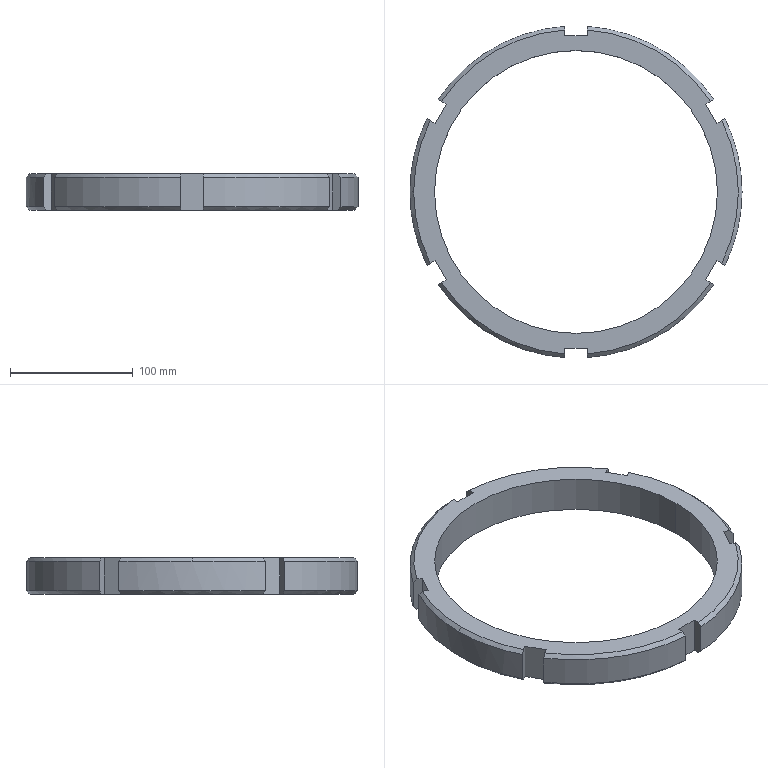Part | SolidWorks | features Chamfer 1, CirPattern 1, ICE 1, Revolution 1 | 1 solid | 43 faces | box 270 x 269.399 x 30 mm | volume 439038 mm3 | plane 20 | cone 14 | cylinder 9 | commonest cylinder face diameters 270 x7 230 x2
STEP:
#1=CARTESIAN_POINT('',(-115.,0.,-30.));
#2=VERTEX_POINT('',#1);
#3=CARTESIAN_POINT('',(115.,0.,-30.));
#4=VERTEX_POINT('',#3);
#5=CARTESIAN_POINT('',(0.,0.,-30.));
#6=DIRECTION('',(0.,0.,1.));
#7=DIRECTION('',(1.,0.,0.));
#8=AXIS2_PLACEMENT_3D('',#5,#6,#7);
#9=CIRCLE('',#8,115.);
#10=EDGE_CURVE('',#2,#4,#9,.T.);
#11=ORIENTED_EDGE('',*,*,#10,.F.);
#12=CARTESIAN_POINT('',(-115.,0.,0.));
#13=VERTEX_POINT('',#12);
#14=CARTESIAN_POINT('',(-115.,0.,0.));
#15=DIRECTION('',(0.,0.,1.));
#16=VECTOR('',#15,1000.);
#17=LINE('',#14,#16);
#18=EDGE_CURVE('',#2,#13,#17,.T.);
#19=ORIENTED_EDGE('',*,*,#18,.T.);
#20=CARTESIAN_POINT('',(115.,0.,0.));
#21=VERTEX_POINT('',#20);
#22=CARTESIAN_POINT('',(0.,0.,0.));
#23=DIRECTION('',(0.,0.,1.));
#24=DIRECTION('',(1.,0.,0.));
#25=AXIS2_PLACEMENT_3D('',#22,#23,#24);
#26=CIRCLE('',#25,115.);
#27=EDGE_CURVE('',#13,#21,#26,.T.);
#28=ORIENTED_EDGE('',*,*,#27,.T.);
#29=CARTESIAN_POINT('',(115.,0.,0.));
#30=DIRECTION('',(0.,0.,1.));
#31=VECTOR('',#30,1000.);
#32=LINE('',#29,#31);
#33=EDGE_CURVE('',#4,#21,#32,.T.);
#34=ORIENTED_EDGE('',*,*,#33,.F.);
#35=EDGE_LOOP('',(#11,#19,#28,#34));
#36=FACE_OUTER_BOUND('',#35,.T.);
#37=CARTESIAN_POINT('',(0.,0.,0.));
#38=DIRECTION('',(0.,0.,1.));
#39=DIRECTION('',(1.,0.,0.));
#40=AXIS2_PLACEMENT_3D('',#37,#38,#39);
#41=CYLINDRICAL_SURFACE('',#40,115.);
#42=ADVANCED_FACE('',(#36),#41,.F.);
#43=CARTESIAN_POINT('',(-132.,0.,0.));
#44=VERTEX_POINT('',#43);
#45=CARTESIAN_POINT('',(-118.549,-58.052,0.));
#46=VERTEX_POINT('',#45);
#47=CARTESIAN_POINT('',(0.,0.,0.));
#48=DIRECTION('',(0.,0.,1.));
#49=DIRECTION('',(-1.,0.,0.));
#50=AXIS2_PLACEMENT_3D('',#47,#48,#49);
#51=CIRCLE('',#50,132.);
#52=EDGE_CURVE('',#44,#46,#51,.T.);
#53=ORIENTED_EDGE('',*,*,#52,.F.);
#54=CARTESIAN_POINT('',(-135.,0.,-3.));
#55=VERTEX_POINT('',#54);
#56=CARTESIAN_POINT('',(-132.,0.,0.));
#57=DIRECTION('',(-0.7071,0.,-0.7071));
#58=VECTOR('',#57,1000.);
#59=LINE('',#56,#58);
#60=EDGE_CURVE('',#44,#55,#59,.T.);
#61=ORIENTED_EDGE('',*,*,#60,.T.);
#62=CARTESIAN_POINT('',(-121.153,-59.556,-3.));
#63=VERTEX_POINT('',#62);
#64=CARTESIAN_POINT('',(0.,0.,-3.));
#65=DIRECTION('',(0.,0.,-1.));
#66=DIRECTION('',(-1.,0.,0.));
#67=AXIS2_PLACEMENT_3D('',#64,#65,#66);
#68=CIRCLE('',#67,135.);
#69=EDGE_CURVE('',#63,#55,#68,.T.);
#70=ORIENTED_EDGE('',*,*,#69,.F.);
#71=CARTESIAN_POINT('',(-118.549,-58.052,0.));
#72=CARTESIAN_POINT('',(-119.417,-58.553,-1.));
#73=CARTESIAN_POINT('',(-120.285,-59.054,-2.));
#74=CARTESIAN_POINT('',(-121.153,-59.556,-3.));
#75=B_SPLINE_CURVE_WITH_KNOTS('',3,(#71,#72,#73,#74),.UNSPECIFIED.,.F.,.F.,(4,4),(0.000000283,0.004248),.UNSPECIFIED.);
#76=EDGE_CURVE('',#46,#63,#75,.T.);
#77=ORIENTED_EDGE('',*,*,#76,.F.);
#78=EDGE_LOOP('',(#53,#61,#70,#77));
#79=FACE_OUTER_BOUND('',#78,.T.);
#80=CARTESIAN_POINT('',(0.,0.,0.));
#81=DIRECTION('',(0.,0.,-1.));
#82=DIRECTION('',(-1.,0.,0.));
#83=AXIS2_PLACEMENT_3D('',#80,#81,#82);
#84=CONICAL_SURFACE('',#83,132.,0.7854);
#85=ADVANCED_FACE('',(#79),#84,.T.);
#86=CARTESIAN_POINT('',(132.,0.,-30.));
#87=VERTEX_POINT('',#86);
#88=CARTESIAN_POINT('',(118.549,-58.052,-30.));
#89=VERTEX_POINT('',#88);
#90=CARTESIAN_POINT('',(0.,0.,-30.));
#91=DIRECTION('',(0.,0.,-1.));
#92=DIRECTION('',(1.,0.,0.));
#93=AXIS2_PLACEMENT_3D('',#90,#91,#92);
#94=CIRCLE('',#93,132.);
#95=EDGE_CURVE('',#87,#89,#94,.T.);
#96=ORIENTED_EDGE('',*,*,#95,.F.);
#97=CARTESIAN_POINT('',(135.,0.,-27.));
#98=VERTEX_POINT('',#97);
#99=CARTESIAN_POINT('',(135.,0.,-27.));
#100=DIRECTION('',(0.7071,0.,0.7071));
#101=VECTOR('',#100,1000.);
#102=LINE('',#99,#101);
#103=EDGE_CURVE('',#87,#98,#102,.T.);
#104=ORIENTED_EDGE('',*,*,#103,.T.);
#105=CARTESIAN_POINT('',(121.153,-59.556,-27.));
#106=VERTEX_POINT('',#105);
#107=CARTESIAN_POINT('',(0.,0.,-27.));
#108=DIRECTION('',(0.,0.,1.));
#109=DIRECTION('',(1.,0.,0.));
#110=AXIS2_PLACEMENT_3D('',#107,#108,#109);
#111=CIRCLE('',#110,135.);
#112=EDGE_CURVE('',#106,#98,#111,.T.);
#113=ORIENTED_EDGE('',*,*,#112,.F.);
#114=CARTESIAN_POINT('',(118.549,-58.052,-30.));
#115=CARTESIAN_POINT('',(119.417,-58.553,-29.));
#116=CARTESIAN_POINT('',(120.285,-59.054,-28.));
#117=CARTESIAN_POINT('',(121.153,-59.556,-27.));
#118=B_SPLINE_CURVE_WITH_KNOTS('',3,(#114,#115,#116,#117),.UNSPECIFIED.,.F.,.F.,(4,4),(0.000000283,0.004248),.UNSPECIFIED.);
#119=EDGE_CURVE('',#89,#106,#118,.T.);
#120=ORIENTED_EDGE('',*,*,#119,.F.);
#121=EDGE_LOOP('',(#96,#104,#113,#120));
#122=FACE_OUTER_BOUND('',#121,.T.);
#123=CARTESIAN_POINT('',(0.,0.,-27.));
#124=DIRECTION('',(0.,0.,1.));
#125=DIRECTION('',(1.,0.,0.));
#126=AXIS2_PLACEMENT_3D('',#123,#124,#125);
#127=CONICAL_SURFACE('',#126,135.,0.7854);
#128=ADVANCED_FACE('',(#122),#127,.T.);
#129=ORIENTED_EDGE('',*,*,#112,.T.);
#130=CARTESIAN_POINT('',(135.,0.,-3.));
#131=VERTEX_POINT('',#130);
#132=CARTESIAN_POINT('',(135.,0.,0.));
#133=DIRECTION('',(0.,0.,1.));
#134=VECTOR('',#133,1000.);
#135=LINE('',#132,#134);
#136=EDGE_CURVE('',#98,#131,#135,.T.);
#137=ORIENTED_EDGE('',*,*,#136,.T.);
#138=CARTESIAN_POINT('',(121.153,-59.556,-3.));
#139=VERTEX_POINT('',#138);
#140=CARTESIAN_POINT('',(0.,0.,-3.));
#141=DIRECTION('',(0.,0.,-1.));
#142=DIRECTION('',(-1.,0.,0.));
#143=AXIS2_PLACEMENT_3D('',#140,#141,#142);
#144=CIRCLE('',#143,135.);
#145=EDGE_CURVE('',#131,#139,#144,.T.);
#146=ORIENTED_EDGE('',*,*,#145,.T.);
#147=CARTESIAN_POINT('',(121.153,-59.556,0.));
#148=DIRECTION('',(0.,0.,-1.));
#149=VECTOR('',#148,1000.);
#150=LINE('',#147,#149);
#151=EDGE_CURVE('',#139,#106,#150,.T.);
#152=ORIENTED_EDGE('',*,*,#151,.T.);
#153=EDGE_LOOP('',(#129,#137,#146,#152));
#154=FACE_OUTER_BOUND('',#153,.T.);
#155=CARTESIAN_POINT('',(0.,0.,0.));
#156=DIRECTION('',(0.,0.,1.));
#157=DIRECTION('',(1.,0.,0.));
#158=AXIS2_PLACEMENT_3D('',#155,#156,#157);
#159=CYLINDRICAL_SURFACE('',#158,135.);
#160=ADVANCED_FACE('',(#154),#159,.T.);
#161=CARTESIAN_POINT('',(-9.,-134.7,-3.));
#162=VERTEX_POINT('',#161);
#163=CARTESIAN_POINT('',(-112.153,-75.144,-3.));
#164=VERTEX_POINT('',#163);
#165=CARTESIAN_POINT('',(0.,0.,-3.));
#166=DIRECTION('',(0.,0.,-1.));
#167=DIRECTION('',(-1.,0.,0.));
#168=AXIS2_PLACEMENT_3D('',#165,#166,#167);
#169=CIRCLE('',#168,135.);
#170=EDGE_CURVE('',#162,#164,#169,.T.);
#171=ORIENTED_EDGE('',*,*,#170,.T.);
#172=CARTESIAN_POINT('',(-112.153,-75.144,-27.));
#173=VERTEX_POINT('',#172);
#174=CARTESIAN_POINT('',(-112.153,-75.144,0.));
#175=DIRECTION('',(0.,0.,-1.));
#176=VECTOR('',#175,1000.);
#177=LINE('',#174,#176);
#178=EDGE_CURVE('',#164,#173,#177,.T.);
#179=ORIENTED_EDGE('',*,*,#178,.T.);
#180=CARTESIAN_POINT('',(-9.,-134.7,-27.));
#181=VERTEX_POINT('',#180);
#182=CARTESIAN_POINT('',(0.,0.,-27.));
#183=DIRECTION('',(0.,0.,1.));
#184=DIRECTION('',(1.,0.,0.));
#185=AXIS2_PLACEMENT_3D('',#182,#183,#184);
#186=CIRCLE('',#185,135.);
#187=EDGE_CURVE('',#173,#181,#186,.T.);
#188=ORIENTED_EDGE('',*,*,#187,.T.);
#189=CARTESIAN_POINT('',(-9.,-134.7,0.));
#190=DIRECTION('',(0.,0.,1.));
#191=VECTOR('',#190,1000.);
#192=LINE('',#189,#191);
#193=EDGE_CURVE('',#181,#162,#192,.T.);
#194=ORIENTED_EDGE('',*,*,#193,.T.);
#195=EDGE_LOOP('',(#171,#179,#188,#194));
#196=FACE_OUTER_BOUND('',#195,.T.);
#197=CARTESIAN_POINT('',(0.,0.,0.));
#198=DIRECTION('',(0.,0.,1.));
#199=DIRECTION('',(1.,0.,0.));
#200=AXIS2_PLACEMENT_3D('',#197,#198,#199);
#201=CYLINDRICAL_SURFACE('',#200,135.);
#202=ADVANCED_FACE('',(#196),#201,.T.);
#203=CARTESIAN_POINT('',(112.153,-75.144,-3.));
#204=VERTEX_POINT('',#203);
#205=CARTESIAN_POINT('',(9.,-134.7,-3.));
#206=VERTEX_POINT('',#205);
#207=CARTESIAN_POINT('',(0.,0.,-3.));
#208=DIRECTION('',(0.,0.,-1.));
#209=DIRECTION('',(-1.,0.,0.));
#210=AXIS2_PLACEMENT_3D('',#207,#208,#209);
#211=CIRCLE('',#210,135.);
#212=EDGE_CURVE('',#204,#206,#211,.T.);
#213=ORIENTED_EDGE('',*,*,#212,.T.);
#214=CARTESIAN_POINT('',(9.,-134.7,-27.));
#215=VERTEX_POINT('',#214);
#216=CARTESIAN_POINT('',(9.,-134.7,0.));
#217=DIRECTION('',(0.,0.,-1.));
#218=VECTOR('',#217,1000.);
#219=LINE('',#216,#218);
#220=EDGE_CURVE('',#206,#215,#219,.T.);
#221=ORIENTED_EDGE('',*,*,#220,.T.);
#222=CARTESIAN_POINT('',(112.153,-75.144,-27.));
#223=VERTEX_POINT('',#222);
#224=CARTESIAN_POINT('',(0.,0.,-27.));
#225=DIRECTION('',(0.,0.,1.));
#226=DIRECTION('',(1.,0.,0.));
#227=AXIS2_PLACEMENT_3D('',#224,#225,#226);
#228=CIRCLE('',#227,135.);
#229=EDGE_CURVE('',#215,#223,#228,.T.);
#230=ORIENTED_EDGE('',*,*,#229,.T.);
#231=CARTESIAN_POINT('',(112.153,-75.144,0.));
#232=DIRECTION('',(0.,0.,1.));
#233=VECTOR('',#232,1000.);
#234=LINE('',#231,#233);
#235=EDGE_CURVE('',#223,#204,#234,.T.);
#236=ORIENTED_EDGE('',*,*,#235,.T.);
#237=EDGE_LOOP('',(#213,#221,#230,#236));
#238=FACE_OUTER_BOUND('',#237,.T.);
#239=CARTESIAN_POINT('',(0.,0.,0.));
#240=DIRECTION('',(0.,0.,1.));
#241=DIRECTION('',(1.,0.,0.));
#242=AXIS2_PLACEMENT_3D('',#239,#240,#241);
#243=CYLINDRICAL_SURFACE('',#242,135.);
#244=ADVANCED_FACE('',(#238),#243,.T.);
#245=ORIENTED_EDGE('',*,*,#136,.F.);
#246=CARTESIAN_POINT('',(121.153,59.556,-27.));
#247=VERTEX_POINT('',#246);
#248=CARTESIAN_POINT('',(0.,0.,-27.));
#249=DIRECTION('',(0.,0.,1.));
#250=DIRECTION('',(1.,0.,0.));
#251=AXIS2_PLACEMENT_3D('',#248,#249,#250);
#252=CIRCLE('',#251,135.);
#253=EDGE_CURVE('',#98,#247,#252,.T.);
#254=ORIENTED_EDGE('',*,*,#253,.T.);
#255=CARTESIAN_POINT('',(121.153,59.556,-3.));
#256=VERTEX_POINT('',#255);
#257=CARTESIAN_POINT('',(121.153,59.556,0.));
#258=DIRECTION('',(0.,0.,1.));
#259=VECTOR('',#258,1000.);
#260=LINE('',#257,#259);
#261=EDGE_CURVE('',#247,#256,#260,.T.);
#262=ORIENTED_EDGE('',*,*,#261,.T.);
#263=CARTESIAN_POINT('',(0.,0.,-3.));
#264=DIRECTION('',(0.,0.,-1.));
#265=DIRECTION('',(-1.,0.,0.));
#266=AXIS2_PLACEMENT_3D('',#263,#264,#265);
#267=CIRCLE('',#266,135.);
#268=EDGE_CURVE('',#256,#131,#267,.T.);
#269=ORIENTED_EDGE('',*,*,#268,.T.);
#270=EDGE_LOOP('',(#245,#254,#262,#269));
#271=FACE_OUTER_BOUND('',#270,.T.);
#272=CARTESIAN_POINT('',(0.,0.,0.));
#273=DIRECTION('',(0.,0.,1.));
#274=DIRECTION('',(1.,0.,0.));
#275=AXIS2_PLACEMENT_3D('',#272,#273,#274);
#276=CYLINDRICAL_SURFACE('',#275,135.);
#277=ADVANCED_FACE('',(#271),#276,.T.);
#278=CARTESIAN_POINT('',(9.,134.7,-3.));
#279=VERTEX_POINT('',#278);
#280=CARTESIAN_POINT('',(112.153,75.144,-3.));
#281=VERTEX_POINT('',#280);
#282=CARTESIAN_POINT('',(0.,0.,-3.));
#283=DIRECTION('',(0.,0.,-1.));
#284=DIRECTION('',(-1.,0.,0.));
#285=AXIS2_PLACEMENT_3D('',#282,#283,#284);
#286=CIRCLE('',#285,135.);
#287=EDGE_CURVE('',#279,#281,#286,.T.);
#288=ORIENTED_EDGE('',*,*,#287,.T.);
#289=CARTESIAN_POINT('',(112.153,75.144,-27.));
#290=VERTEX_POINT('',#289);
#291=CARTESIAN_POINT('',(112.153,75.144,0.));
#292=DIRECTION('',(0.,0.,-1.));
#293=VECTOR('',#292,1000.);
#294=LINE('',#291,#293);
#295=EDGE_CURVE('',#281,#290,#294,.T.);
#296=ORIENTED_EDGE('',*,*,#295,.T.);
#297=CARTESIAN_POINT('',(9.,134.7,-27.));
#298=VERTEX_POINT('',#297);
#299=CARTESIAN_POINT('',(0.,0.,-27.));
#300=DIRECTION('',(0.,0.,1.));
#301=DIRECTION('',(1.,0.,0.));
#302=AXIS2_PLACEMENT_3D('',#299,#300,#301);
#303=CIRCLE('',#302,135.);
#304=EDGE_CURVE('',#290,#298,#303,.T.);
#305=ORIENTED_EDGE('',*,*,#304,.T.);
#306=CARTESIAN_POINT('',(9.,134.7,0.));
#307=DIRECTION('',(0.,0.,1.));
#308=VECTOR('',#307,1000.);
#309=LINE('',#306,#308);
#310=EDGE_CURVE('',#298,#279,#309,.T.);
#311=ORIENTED_EDGE('',*,*,#310,.T.);
#312=EDGE_LOOP('',(#288,#296,#305,#311));
#313=FACE_OUTER_BOUND('',#312,.T.);
#314=CARTESIAN_POINT('',(0.,0.,0.));
#315=DIRECTION('',(0.,0.,1.));
#316=DIRECTION('',(1.,0.,0.));
#317=AXIS2_PLACEMENT_3D('',#314,#315,#316);
#318=CYLINDRICAL_SURFACE('',#317,135.);
#319=ADVANCED_FACE('',(#313),#318,.T.);
#320=CARTESIAN_POINT('',(-109.549,-73.641,-30.));
#321=VERTEX_POINT('',#320);
#322=CARTESIAN_POINT('',(-109.549,-73.641,-30.));
#323=CARTESIAN_POINT('',(-110.417,-74.142,-29.));
#324=CARTESIAN_POINT('',(-111.285,-74.643,-28.));
#325=CARTESIAN_POINT('',(-112.153,-75.144,-27.));
#326=B_SPLINE_CURVE_WITH_KNOTS('',3,(#322,#323,#324,#325),.UNSPECIFIED.,.F.,.F.,(4,4),(0.000000283,0.004248),.UNSPECIFIED.);
#327=EDGE_CURVE('',#321,#173,#326,.T.);
#328=ORIENTED_EDGE('',*,*,#327,.F.);
#329=CARTESIAN_POINT('',(-9.,-131.693,-30.));
#330=VERTEX_POINT('',#329);
#331=CARTESIAN_POINT('',(0.,0.,-30.));
#332=DIRECTION('',(0.,0.,-1.));
#333=DIRECTION('',(1.,0.,0.));
#334=AXIS2_PLACEMENT_3D('',#331,#332,#333);
#335=CIRCLE('',#334,132.);
#336=EDGE_CURVE('',#330,#321,#335,.T.);
#337=ORIENTED_EDGE('',*,*,#336,.F.);
#338=CARTESIAN_POINT('',(-9.,-134.7,-27.));
#339=CARTESIAN_POINT('',(-9.,-134.333,-27.366));
#340=CARTESIAN_POINT('',(-9.,-133.966,-27.732));
#341=CARTESIAN_POINT('',(-9.,-133.599,-28.098));
#342=CARTESIAN_POINT('',(-9.,-132.964,-28.732));
#343=CARTESIAN_POINT('',(-9.,-132.328,-29.366));
#344=CARTESIAN_POINT('',(-9.,-131.693,-30.));
#345=B_SPLINE_CURVE_WITH_KNOTS('',3,(#338,#339,#340,#341,#342,#343,#344),.UNSPECIFIED.,.F.,.F.,(4,3,4),(0.01543,0.01698,0.01967),.UNSPECIFIED.);
#346=EDGE_CURVE('',#181,#330,#345,.T.);
#347=ORIENTED_EDGE('',*,*,#346,.F.);
#348=ORIENTED_EDGE('',*,*,#187,.F.);
#349=EDGE_LOOP('',(#328,#337,#347,#348));
#350=FACE_OUTER_BOUND('',#349,.T.);
#351=CARTESIAN_POINT('',(0.,0.,-27.));
#352=DIRECTION('',(0.,0.,1.));
#353=DIRECTION('',(1.,0.,0.));
#354=AXIS2_PLACEMENT_3D('',#351,#352,#353);
#355=CONICAL_SURFACE('',#354,135.,0.7854);
#356=ADVANCED_FACE('',(#350),#355,.T.);
#357=CARTESIAN_POINT('',(9.,-131.693,-30.));
#358=VERTEX_POINT('',#357);
#359=CARTESIAN_POINT('',(9.,-131.693,-30.));
#360=CARTESIAN_POINT('',(9.,-132.328,-29.366));
#361=CARTESIAN_POINT('',(9.,-132.964,-28.732));
#362=CARTESIAN_POINT('',(9.,-133.599,-28.098));
#363=CARTESIAN_POINT('',(9.,-133.966,-27.732));
#364=CARTESIAN_POINT('',(9.,-134.333,-27.366));
#365=CARTESIAN_POINT('',(9.,-134.7,-27.));
#366=B_SPLINE_CURVE_WITH_KNOTS('',3,(#359,#360,#361,#362,#363,#364,#365),.UNSPECIFIED.,.F.,.F.,(4,3,4),(0.01429,0.01698,0.01854),.UNSPECIFIED.);
#367=EDGE_CURVE('',#358,#215,#366,.T.);
#368=ORIENTED_EDGE('',*,*,#367,.F.);
#369=CARTESIAN_POINT('',(109.549,-73.641,-30.));
#370=VERTEX_POINT('',#369);
#371=CARTESIAN_POINT('',(0.,0.,-30.));
#372=DIRECTION('',(0.,0.,-1.));
#373=DIRECTION('',(1.,0.,0.));
#374=AXIS2_PLACEMENT_3D('',#371,#372,#373);
#375=CIRCLE('',#374,132.);
#376=EDGE_CURVE('',#370,#358,#375,.T.);
#377=ORIENTED_EDGE('',*,*,#376,.F.);
#378=CARTESIAN_POINT('',(112.153,-75.144,-27.));
#379=CARTESIAN_POINT('',(111.285,-74.643,-28.));
#380=CARTESIAN_POINT('',(110.417,-74.142,-29.));
#381=CARTESIAN_POINT('',(109.549,-73.641,-30.));
#382=B_SPLINE_CURVE_WITH_KNOTS('',3,(#378,#379,#380,#381),.UNSPECIFIED.,.F.,.F.,(4,4),(0.000000283,0.004248),.UNSPECIFIED.);
#383=EDGE_CURVE('',#223,#370,#382,.T.);
#384=ORIENTED_EDGE('',*,*,#383,.F.);
#385=ORIENTED_EDGE('',*,*,#229,.F.);
#386=EDGE_LOOP('',(#368,#377,#384,#385));
#387=FACE_OUTER_BOUND('',#386,.T.);
#388=CARTESIAN_POINT('',(0.,0.,-27.));
#389=DIRECTION('',(0.,0.,1.));
#390=DIRECTION('',(1.,0.,0.));
#391=AXIS2_PLACEMENT_3D('',#388,#389,#390);
#392=CONICAL_SURFACE('',#391,135.,0.7854);
#393=ADVANCED_FACE('',(#387),#392,.T.);
#394=ORIENTED_EDGE('',*,*,#103,.F.);
#395=CARTESIAN_POINT('',(118.549,58.052,-30.));
#396=VERTEX_POINT('',#395);
#397=CARTESIAN_POINT('',(0.,0.,-30.));
#398=DIRECTION('',(0.,0.,-1.));
#399=DIRECTION('',(1.,0.,0.));
#400=AXIS2_PLACEMENT_3D('',#397,#398,#399);
#401=CIRCLE('',#400,132.);
#402=EDGE_CURVE('',#396,#87,#401,.T.);
#403=ORIENTED_EDGE('',*,*,#402,.F.);
#404=CARTESIAN_POINT('',(121.153,59.556,-27.));
#405=CARTESIAN_POINT('',(120.285,59.054,-28.));
#406=CARTESIAN_POINT('',(119.417,58.553,-29.));
#407=CARTESIAN_POINT('',(118.549,58.052,-30.));
#408=B_SPLINE_CURVE_WITH_KNOTS('',3,(#404,#405,#406,#407),.UNSPECIFIED.,.F.,.F.,(4,4),(0.000000283,0.004248),.UNSPECIFIED.);
#409=EDGE_CURVE('',#247,#396,#408,.T.);
#410=ORIENTED_EDGE('',*,*,#409,.F.);
#411=ORIENTED_EDGE('',*,*,#253,.F.);
#412=EDGE_LOOP('',(#394,#403,#410,#411));
#413=FACE_OUTER_BOUND('',#412,.T.);
#414=CARTESIAN_POINT('',(0.,0.,-27.));
#415=DIRECTION('',(0.,0.,1.));
#416=DIRECTION('',(1.,0.,0.));
#417=AXIS2_PLACEMENT_3D('',#414,#415,#416);
#418=CONICAL_SURFACE('',#417,135.,0.7854);
#419=ADVANCED_FACE('',(#413),#418,.T.);
#420=CARTESIAN_POINT('',(109.549,73.641,-30.));
#421=VERTEX_POINT('',#420);
#422=CARTESIAN_POINT('',(109.549,73.641,-30.));
#423=CARTESIAN_POINT('',(110.417,74.142,-29.));
#424=CARTESIAN_POINT('',(111.285,74.643,-28.));
#425=CARTESIAN_POINT('',(112.153,75.144,-27.));
#426=B_SPLINE_CURVE_WITH_KNOTS('',3,(#422,#423,#424,#425),.UNSPECIFIED.,.F.,.F.,(4,4),(0.000000283,0.004248),.UNSPECIFIED.);
#427=EDGE_CURVE('',#421,#290,#426,.T.);
#428=ORIENTED_EDGE('',*,*,#427,.F.);
#429=CARTESIAN_POINT('',(9.,131.693,-30.));
#430=VERTEX_POINT('',#429);
#431=CARTESIAN_POINT('',(0.,0.,-30.));
#432=DIRECTION('',(0.,0.,-1.));
#433=DIRECTION('',(1.,0.,0.));
#434=AXIS2_PLACEMENT_3D('',#431,#432,#433);
#435=CIRCLE('',#434,132.);
#436=EDGE_CURVE('',#430,#421,#435,.T.);
#437=ORIENTED_EDGE('',*,*,#436,.F.);
#438=CARTESIAN_POINT('',(9.,134.7,-27.));
#439=CARTESIAN_POINT('',(9.,133.999,-27.699));
#440=CARTESIAN_POINT('',(9.,133.298,-28.399));
#441=CARTESIAN_POINT('',(9.,132.597,-29.098));
#442=CARTESIAN_POINT('',(9.,132.295,-29.399));
#443=CARTESIAN_POINT('',(9.,131.994,-29.699));
#444=CARTESIAN_POINT('',(9.,131.693,-30.));
#445=B_SPLINE_CURVE_WITH_KNOTS('',3,(#438,#439,#440,#441,#442,#443,#444),.UNSPECIFIED.,.F.,.F.,(4,3,4),(0.01401,0.01698,0.01826),.UNSPECIFIED.);
#446=EDGE_CURVE('',#298,#430,#445,.T.);
#447=ORIENTED_EDGE('',*,*,#446,.F.);
#448=ORIENTED_EDGE('',*,*,#304,.F.);
#449=EDGE_LOOP('',(#428,#437,#447,#448));
#450=FACE_OUTER_BOUND('',#449,.T.);
#451=CARTESIAN_POINT('',(0.,0.,-27.));
#452=DIRECTION('',(0.,0.,1.));
#453=DIRECTION('',(1.,0.,0.));
#454=AXIS2_PLACEMENT_3D('',#451,#452,#453);
#455=CONICAL_SURFACE('',#454,135.,0.7854);
#456=ADVANCED_FACE('',(#450),#455,.T.);
#457=CARTESIAN_POINT('',(-109.549,-73.641,0.));
#458=VERTEX_POINT('',#457);
#459=CARTESIAN_POINT('',(-112.153,-75.144,-3.));
#460=CARTESIAN_POINT('',(-111.285,-74.643,-2.));
#461=CARTESIAN_POINT('',(-110.417,-74.142,-1.));
#462=CARTESIAN_POINT('',(-109.549,-73.641,0.));
#463=B_SPLINE_CURVE_WITH_KNOTS('',3,(#459,#460,#461,#462),.UNSPECIFIED.,.F.,.F.,(4,4),(0.000000283,0.004248),.UNSPECIFIED.);
#464=EDGE_CURVE('',#164,#458,#463,.T.);
#465=ORIENTED_EDGE('',*,*,#464,.F.);
#466=ORIENTED_EDGE('',*,*,#170,.F.);
#467=CARTESIAN_POINT('',(-9.,-131.693,0.));
#468=VERTEX_POINT('',#467);
#469=CARTESIAN_POINT('',(-9.,-131.693,0.));
#470=CARTESIAN_POINT('',(-9.,-132.328,-0.6339));
#471=CARTESIAN_POINT('',(-9.,-132.964,-1.268));
#472=CARTESIAN_POINT('',(-9.,-133.599,-1.902));
#473=CARTESIAN_POINT('',(-9.,-133.966,-2.268));
#474=CARTESIAN_POINT('',(-9.,-134.333,-2.634));
#475=CARTESIAN_POINT('',(-9.,-134.7,-3.));
#476=B_SPLINE_CURVE_WITH_KNOTS('',3,(#469,#470,#471,#472,#473,#474,#475),.UNSPECIFIED.,.F.,.F.,(4,3,4),(0.01429,0.01698,0.01854),.UNSPECIFIED.);
#477=EDGE_CURVE('',#468,#162,#476,.T.);
#478=ORIENTED_EDGE('',*,*,#477,.F.);
#479=CARTESIAN_POINT('',(0.,0.,0.));
#480=DIRECTION('',(0.,0.,1.));
#481=DIRECTION('',(-1.,0.,0.));
#482=AXIS2_PLACEMENT_3D('',#479,#480,#481);
#483=CIRCLE('',#482,132.);
#484=EDGE_CURVE('',#458,#468,#483,.T.);
#485=ORIENTED_EDGE('',*,*,#484,.F.);
#486=EDGE_LOOP('',(#465,#466,#478,#485));
#487=FACE_OUTER_BOUND('',#486,.T.);
#488=CARTESIAN_POINT('',(0.,0.,0.));
#489=DIRECTION('',(0.,0.,-1.));
#490=DIRECTION('',(-1.,0.,0.));
#491=AXIS2_PLACEMENT_3D('',#488,#489,#490);
#492=CONICAL_SURFACE('',#491,132.,0.7854);
#493=ADVANCED_FACE('',(#487),#492,.T.);
#494=CARTESIAN_POINT('',(9.,-131.693,0.));
#495=VERTEX_POINT('',#494);
#496=CARTESIAN_POINT('',(9.,-134.7,-3.));
#497=CARTESIAN_POINT('',(9.,-134.333,-2.634));
#498=CARTESIAN_POINT('',(9.,-133.966,-2.268));
#499=CARTESIAN_POINT('',(9.,-133.599,-1.902));
#500=CARTESIAN_POINT('',(9.,-132.964,-1.268));
#501=CARTESIAN_POINT('',(9.,-132.328,-0.6339));
#502=CARTESIAN_POINT('',(9.,-131.693,0.));
#503=B_SPLINE_CURVE_WITH_KNOTS('',3,(#496,#497,#498,#499,#500,#501,#502),.UNSPECIFIED.,.F.,.F.,(4,3,4),(0.01543,0.01698,0.01967),.UNSPECIFIED.);
#504=EDGE_CURVE('',#206,#495,#503,.T.);
#505=ORIENTED_EDGE('',*,*,#504,.F.);
#506=ORIENTED_EDGE('',*,*,#212,.F.);
#507=CARTESIAN_POINT('',(109.549,-73.641,0.));
#508=VERTEX_POINT('',#507);
#509=CARTESIAN_POINT('',(109.549,-73.641,0.));
#510=CARTESIAN_POINT('',(110.417,-74.142,-1.));
#511=CARTESIAN_POINT('',(111.285,-74.643,-2.));
#512=CARTESIAN_POINT('',(112.153,-75.144,-3.));
#513=B_SPLINE_CURVE_WITH_KNOTS('',3,(#509,#510,#511,#512),.UNSPECIFIED.,.F.,.F.,(4,4),(0.000000283,0.004248),.UNSPECIFIED.);
#514=EDGE_CURVE('',#508,#204,#513,.T.);
#515=ORIENTED_EDGE('',*,*,#514,.F.);
#516=CARTESIAN_POINT('',(0.,0.,0.));
#517=DIRECTION('',(0.,0.,1.));
#518=DIRECTION('',(-1.,0.,0.));
#519=AXIS2_PLACEMENT_3D('',#516,#517,#518);
#520=CIRCLE('',#519,132.);
#521=EDGE_CURVE('',#495,#508,#520,.T.);
#522=ORIENTED_EDGE('',*,*,#521,.F.);
#523=EDGE_LOOP('',(#505,#506,#515,#522));
#524=FACE_OUTER_BOUND('',#523,.T.);
#525=CARTESIAN_POINT('',(0.,0.,0.));
#526=DIRECTION('',(0.,0.,-1.));
#527=DIRECTION('',(-1.,0.,0.));
#528=AXIS2_PLACEMENT_3D('',#525,#526,#527);
#529=CONICAL_SURFACE('',#528,132.,0.7854);
#530=ADVANCED_FACE('',(#524),#529,.T.);
#531=CARTESIAN_POINT('',(118.549,-58.052,0.));
#532=VERTEX_POINT('',#531);
#533=CARTESIAN_POINT('',(121.153,-59.556,-3.));
#534=CARTESIAN_POINT('',(120.285,-59.054,-2.));
#535=CARTESIAN_POINT('',(119.417,-58.553,-1.));
#536=CARTESIAN_POINT('',(118.549,-58.052,0.));
#537=B_SPLINE_CURVE_WITH_KNOTS('',3,(#533,#534,#535,#536),.UNSPECIFIED.,.F.,.F.,(4,4),(0.000000283,0.004248),.UNSPECIFIED.);
#538=EDGE_CURVE('',#139,#532,#537,.T.);
#539=ORIENTED_EDGE('',*,*,#538,.F.);
#540=ORIENTED_EDGE('',*,*,#145,.F.);
#541=ORIENTED_EDGE('',*,*,#268,.F.);
#542=CARTESIAN_POINT('',(118.549,58.052,0.));
#543=VERTEX_POINT('',#542);
#544=CARTESIAN_POINT('',(118.549,58.052,0.));
#545=CARTESIAN_POINT('',(119.417,58.553,-1.));
#546=CARTESIAN_POINT('',(120.285,59.054,-2.));
#547=CARTESIAN_POINT('',(121.153,59.556,-3.));
#548=B_SPLINE_CURVE_WITH_KNOTS('',3,(#544,#545,#546,#547),.UNSPECIFIED.,.F.,.F.,(4,4),(0.000000283,0.004248),.UNSPECIFIED.);
#549=EDGE_CURVE('',#543,#256,#548,.T.);
#550=ORIENTED_EDGE('',*,*,#549,.F.);
#551=CARTESIAN_POINT('',(0.,0.,0.));
#552=DIRECTION('',(0.,0.,1.));
#553=DIRECTION('',(-1.,0.,0.));
#554=AXIS2_PLACEMENT_3D('',#551,#552,#553);
#555=CIRCLE('',#554,132.);
#556=EDGE_CURVE('',#532,#543,#555,.T.);
#557=ORIENTED_EDGE('',*,*,#556,.F.);
#558=EDGE_LOOP('',(#539,#540,#541,#550,#557));
#559=FACE_OUTER_BOUND('',#558,.T.);
#560=CARTESIAN_POINT('',(0.,0.,0.));
#561=DIRECTION('',(0.,0.,-1.));
#562=DIRECTION('',(-1.,0.,0.));
#563=AXIS2_PLACEMENT_3D('',#560,#561,#562);
#564=CONICAL_SURFACE('',#563,132.,0.7854);
#565=ADVANCED_FACE('',(#559),#564,.T.);
#566=CARTESIAN_POINT('',(109.549,73.641,0.));
#567=VERTEX_POINT('',#566);
#568=CARTESIAN_POINT('',(112.153,75.144,-3.));
#569=CARTESIAN_POINT('',(111.285,74.643,-2.));
#570=CARTESIAN_POINT('',(110.417,74.142,-1.));
#571=CARTESIAN_POINT('',(109.549,73.641,0.));
#572=B_SPLINE_CURVE_WITH_KNOTS('',3,(#568,#569,#570,#571),.UNSPECIFIED.,.F.,.F.,(4,4),(0.000000283,0.004248),.UNSPECIFIED.);
#573=EDGE_CURVE('',#281,#567,#572,.T.);
#574=ORIENTED_EDGE('',*,*,#573,.F.);
#575=ORIENTED_EDGE('',*,*,#287,.F.);
#576=CARTESIAN_POINT('',(9.,131.693,0.));
#577=VERTEX_POINT('',#576);
#578=CARTESIAN_POINT('',(9.,131.693,0.));
#579=CARTESIAN_POINT('',(9.,131.994,-0.3006));
#580=CARTESIAN_POINT('',(9.,132.295,-0.6012));
#581=CARTESIAN_POINT('',(9.,132.597,-0.9019));
#582=CARTESIAN_POINT('',(9.,133.298,-1.601));
#583=CARTESIAN_POINT('',(9.,133.999,-2.301));
#584=CARTESIAN_POINT('',(9.,134.7,-3.));
#585=B_SPLINE_CURVE_WITH_KNOTS('',3,(#578,#579,#580,#581,#582,#583,#584),.UNSPECIFIED.,.F.,.F.,(4,3,4),(0.0157,0.01698,0.01995),.UNSPECIFIED.);
#586=EDGE_CURVE('',#577,#279,#585,.T.);
#587=ORIENTED_EDGE('',*,*,#586,.F.);
#588=CARTESIAN_POINT('',(0.,0.,0.));
#589=DIRECTION('',(0.,0.,1.));
#590=DIRECTION('',(-1.,0.,0.));
#591=AXIS2_PLACEMENT_3D('',#588,#589,#590);
#592=CIRCLE('',#591,132.);
#593=EDGE_CURVE('',#567,#577,#592,.T.);
#594=ORIENTED_EDGE('',*,*,#593,.F.);
#595=EDGE_LOOP('',(#574,#575,#587,#594));
#596=FACE_OUTER_BOUND('',#595,.T.);
#597=CARTESIAN_POINT('',(0.,0.,0.));
#598=DIRECTION('',(0.,0.,-1.));
#599=DIRECTION('',(-1.,0.,0.));
#600=AXIS2_PLACEMENT_3D('',#597,#598,#599);
#601=CONICAL_SURFACE('',#600,132.,0.7854);
#602=ADVANCED_FACE('',(#596),#601,.T.);
#603=CARTESIAN_POINT('',(-121.153,59.556,-27.));
#604=VERTEX_POINT('',#603);
#605=CARTESIAN_POINT('',(-121.153,-59.556,-27.));
#606=VERTEX_POINT('',#605);
#607=CARTESIAN_POINT('',(0.,0.,-27.));
#608=DIRECTION('',(0.,0.,1.));
#609=DIRECTION('',(1.,0.,0.));
#610=AXIS2_PLACEMENT_3D('',#607,#608,#609);
#611=CIRCLE('',#610,135.);
#612=EDGE_CURVE('',#604,#606,#611,.T.);
#613=ORIENTED_EDGE('',*,*,#612,.T.);
#614=CARTESIAN_POINT('',(-121.153,-59.556,0.));
#615=DIRECTION('',(0.,0.,1.));
#616=VECTOR('',#615,1000.);
#617=LINE('',#614,#616);
#618=EDGE_CURVE('',#606,#63,#617,.T.);
#619=ORIENTED_EDGE('',*,*,#618,.T.);
#620=ORIENTED_EDGE('',*,*,#69,.T.);
#621=CARTESIAN_POINT('',(-121.153,59.556,-3.));
#622=VERTEX_POINT('',#621);
#623=CARTESIAN_POINT('',(0.,0.,-3.));
#624=DIRECTION('',(0.,0.,-1.));
#625=DIRECTION('',(-1.,0.,0.));
#626=AXIS2_PLACEMENT_3D('',#623,#624,#625);
#627=CIRCLE('',#626,135.);
#628=EDGE_CURVE('',#55,#622,#627,.T.);
#629=ORIENTED_EDGE('',*,*,#628,.T.);
#630=CARTESIAN_POINT('',(-121.153,59.556,0.));
#631=DIRECTION('',(0.,0.,-1.));
#632=VECTOR('',#631,1000.);
#633=LINE('',#630,#632);
#634=EDGE_CURVE('',#622,#604,#633,.T.);
#635=ORIENTED_EDGE('',*,*,#634,.T.);
#636=EDGE_LOOP('',(#613,#619,#620,#629,#635));
#637=FACE_OUTER_BOUND('',#636,.T.);
#638=CARTESIAN_POINT('',(0.,0.,0.));
#639=DIRECTION('',(0.,0.,1.));
#640=DIRECTION('',(1.,0.,0.));
#641=AXIS2_PLACEMENT_3D('',#638,#639,#640);
#642=CYLINDRICAL_SURFACE('',#641,135.);
#643=ADVANCED_FACE('',(#637),#642,.T.);
#644=CARTESIAN_POINT('',(-118.549,-58.052,-30.));
#645=VERTEX_POINT('',#644);
#646=CARTESIAN_POINT('',(-121.153,-59.556,-27.));
#647=CARTESIAN_POINT('',(-120.285,-59.054,-28.));
#648=CARTESIAN_POINT('',(-119.417,-58.553,-29.));
#649=CARTESIAN_POINT('',(-118.549,-58.052,-30.));
#650=B_SPLINE_CURVE_WITH_KNOTS('',3,(#646,#647,#648,#649),.UNSPECIFIED.,.F.,.F.,(4,4),(0.000000283,0.004248),.UNSPECIFIED.);
#651=EDGE_CURVE('',#606,#645,#650,.T.);
#652=ORIENTED_EDGE('',*,*,#651,.F.);
#653=ORIENTED_EDGE('',*,*,#612,.F.);
#654=CARTESIAN_POINT('',(-118.549,58.052,-30.));
#655=VERTEX_POINT('',#654);
#656=CARTESIAN_POINT('',(-118.549,58.052,-30.));
#657=CARTESIAN_POINT('',(-119.417,58.553,-29.));
#658=CARTESIAN_POINT('',(-120.285,59.054,-28.));
#659=CARTESIAN_POINT('',(-121.153,59.556,-27.));
#660=B_SPLINE_CURVE_WITH_KNOTS('',3,(#656,#657,#658,#659),.UNSPECIFIED.,.F.,.F.,(4,4),(0.000000283,0.004248),.UNSPECIFIED.);
#661=EDGE_CURVE('',#655,#604,#660,.T.);
#662=ORIENTED_EDGE('',*,*,#661,.F.);
#663=CARTESIAN_POINT('',(0.,0.,-30.));
#664=DIRECTION('',(0.,0.,-1.));
#665=DIRECTION('',(1.,0.,0.));
#666=AXIS2_PLACEMENT_3D('',#663,#664,#665);
#667=CIRCLE('',#666,132.);
#668=EDGE_CURVE('',#645,#655,#667,.T.);
#669=ORIENTED_EDGE('',*,*,#668,.F.);
#670=EDGE_LOOP('',(#652,#653,#662,#669));
#671=FACE_OUTER_BOUND('',#670,.T.);
#672=CARTESIAN_POINT('',(0.,0.,-27.));
#673=DIRECTION('',(0.,0.,1.));
#674=DIRECTION('',(1.,0.,0.));
#675=AXIS2_PLACEMENT_3D('',#672,#673,#674);
#676=CONICAL_SURFACE('',#675,135.,0.7854);
#677=ADVANCED_FACE('',(#671),#676,.T.);
#678=ORIENTED_EDGE('',*,*,#60,.F.);
#679=CARTESIAN_POINT('',(-118.549,58.052,0.));
#680=VERTEX_POINT('',#679);
#681=CARTESIAN_POINT('',(0.,0.,0.));
#682=DIRECTION('',(0.,0.,1.));
#683=DIRECTION('',(-1.,0.,0.));
#684=AXIS2_PLACEMENT_3D('',#681,#682,#683);
#685=CIRCLE('',#684,132.);
#686=EDGE_CURVE('',#680,#44,#685,.T.);
#687=ORIENTED_EDGE('',*,*,#686,.F.);
#688=CARTESIAN_POINT('',(-121.153,59.556,-3.));
#689=CARTESIAN_POINT('',(-120.285,59.054,-2.));
#690=CARTESIAN_POINT('',(-119.417,58.553,-1.));
#691=CARTESIAN_POINT('',(-118.549,58.052,0.));
#692=B_SPLINE_CURVE_WITH_KNOTS('',3,(#688,#689,#690,#691),.UNSPECIFIED.,.F.,.F.,(4,4),(0.000000283,0.004248),.UNSPECIFIED.);
#693=EDGE_CURVE('',#622,#680,#692,.T.);
#694=ORIENTED_EDGE('',*,*,#693,.F.);
#695=ORIENTED_EDGE('',*,*,#628,.F.);
#696=EDGE_LOOP('',(#678,#687,#694,#695));
#697=FACE_OUTER_BOUND('',#696,.T.);
#698=CARTESIAN_POINT('',(0.,0.,0.));
#699=DIRECTION('',(0.,0.,-1.));
#700=DIRECTION('',(-1.,0.,0.));
#701=AXIS2_PLACEMENT_3D('',#698,#699,#700);
#702=CONICAL_SURFACE('',#701,132.,0.7854);
#703=ADVANCED_FACE('',(#697),#702,.T.);
#704=CARTESIAN_POINT('',(-105.485,-71.294,0.));
#705=VERTEX_POINT('',#704);
#706=CARTESIAN_POINT('',(-114.485,-55.706,0.));
#707=VERTEX_POINT('',#706);
#708=CARTESIAN_POINT('',(-114.485,-55.706,0.));
#709=DIRECTION('',(-0.5,0.866,0.));
#710=VECTOR('',#709,1000.);
#711=LINE('',#708,#710);
#712=EDGE_CURVE('',#705,#707,#711,.T.);
#713=ORIENTED_EDGE('',*,*,#712,.F.);
#714=CARTESIAN_POINT('',(-105.485,-71.294,0.));
#715=DIRECTION('',(0.866,0.5,0.));
#716=VECTOR('',#715,1000.);
#717=LINE('',#714,#716);
#718=EDGE_CURVE('',#458,#705,#717,.T.);
#719=ORIENTED_EDGE('',*,*,#718,.F.);
#720=ORIENTED_EDGE('',*,*,#484,.T.);
#721=CARTESIAN_POINT('',(-9.,-127.,0.));
#722=VERTEX_POINT('',#721);
#723=CARTESIAN_POINT('',(-9.,-127.,0.));
#724=DIRECTION('',(0.,-1.,0.));
#725=VECTOR('',#724,1000.);
#726=LINE('',#723,#725);
#727=EDGE_CURVE('',#722,#468,#726,.T.);
#728=ORIENTED_EDGE('',*,*,#727,.F.);
#729=CARTESIAN_POINT('',(9.,-127.,0.));
#730=VERTEX_POINT('',#729);
#731=CARTESIAN_POINT('',(-9.,-127.,0.));
#732=DIRECTION('',(-1.,0.,0.));
#733=VECTOR('',#732,1000.);
#734=LINE('',#731,#733);
#735=EDGE_CURVE('',#730,#722,#734,.T.);
#736=ORIENTED_EDGE('',*,*,#735,.F.);
#737=CARTESIAN_POINT('',(9.,-127.,0.));
#738=DIRECTION('',(0.,1.,0.));
#739=VECTOR('',#738,1000.);
#740=LINE('',#737,#739);
#741=EDGE_CURVE('',#495,#730,#740,.T.);
#742=ORIENTED_EDGE('',*,*,#741,.F.);
#743=ORIENTED_EDGE('',*,*,#521,.T.);
#744=CARTESIAN_POINT('',(105.485,-71.294,0.));
#745=VERTEX_POINT('',#744);
#746=CARTESIAN_POINT('',(105.485,-71.294,0.));
#747=DIRECTION('',(0.866,-0.5,0.));
#748=VECTOR('',#747,1000.);
#749=LINE('',#746,#748);
#750=EDGE_CURVE('',#745,#508,#749,.T.);
#751=ORIENTED_EDGE('',*,*,#750,.F.);
#752=CARTESIAN_POINT('',(114.485,-55.706,0.));
#753=VERTEX_POINT('',#752);
#754=CARTESIAN_POINT('',(105.485,-71.294,0.));
#755=DIRECTION('',(-0.5,-0.866,0.));
#756=VECTOR('',#755,1000.);
#757=LINE('',#754,#756);
#758=EDGE_CURVE('',#753,#745,#757,.T.);
#759=ORIENTED_EDGE('',*,*,#758,.F.);
#760=CARTESIAN_POINT('',(114.485,-55.706,0.));
#761=DIRECTION('',(-0.866,0.5,0.));
#762=VECTOR('',#761,1000.);
#763=LINE('',#760,#762);
#764=EDGE_CURVE('',#532,#753,#763,.T.);
#765=ORIENTED_EDGE('',*,*,#764,.F.);
#766=ORIENTED_EDGE('',*,*,#556,.T.);
#767=CARTESIAN_POINT('',(114.485,55.706,0.));
#768=VERTEX_POINT('',#767);
#769=CARTESIAN_POINT('',(114.485,55.706,0.));
#770=DIRECTION('',(0.866,0.5,0.));
#771=VECTOR('',#770,1000.);
#772=LINE('',#769,#771);
#773=EDGE_CURVE('',#768,#543,#772,.T.);
#774=ORIENTED_EDGE('',*,*,#773,.F.);
#775=CARTESIAN_POINT('',(105.485,71.294,0.));
#776=VERTEX_POINT('',#775);
#777=CARTESIAN_POINT('',(114.485,55.706,0.));
#778=DIRECTION('',(0.5,-0.866,0.));
#779=VECTOR('',#778,1000.);
#780=LINE('',#777,#779);
#781=EDGE_CURVE('',#776,#768,#780,.T.);
#782=ORIENTED_EDGE('',*,*,#781,.F.);
#783=CARTESIAN_POINT('',(105.485,71.294,0.));
#784=DIRECTION('',(-0.866,-0.5,0.));
#785=VECTOR('',#784,1000.);
#786=LINE('',#783,#785);
#787=EDGE_CURVE('',#567,#776,#786,.T.);
#788=ORIENTED_EDGE('',*,*,#787,.F.);
#789=ORIENTED_EDGE('',*,*,#593,.T.);
#790=CARTESIAN_POINT('',(9.,127.,0.));
#791=VERTEX_POINT('',#790);
#792=CARTESIAN_POINT('',(9.,127.,0.));
#793=DIRECTION('',(0.,1.,0.));
#794=VECTOR('',#793,1000.);
#795=LINE('',#792,#794);
#796=EDGE_CURVE('',#791,#577,#795,.T.);
#797=ORIENTED_EDGE('',*,*,#796,.F.);
#798=CARTESIAN_POINT('',(-9.,127.,0.));
#799=VERTEX_POINT('',#798);
#800=CARTESIAN_POINT('',(9.,127.,0.));
#801=DIRECTION('',(1.,0.,0.));
#802=VECTOR('',#801,1000.);
#803=LINE('',#800,#802);
#804=EDGE_CURVE('',#799,#791,#803,.T.);
#805=ORIENTED_EDGE('',*,*,#804,.F.);
#806=CARTESIAN_POINT('',(-9.,131.693,0.));
#807=VERTEX_POINT('',#806);
#808=CARTESIAN_POINT('',(-9.,127.,0.));
#809=DIRECTION('',(0.,-1.,0.));
#810=VECTOR('',#809,1000.);
#811=LINE('',#808,#810);
#812=EDGE_CURVE('',#807,#799,#811,.T.);
#813=ORIENTED_EDGE('',*,*,#812,.F.);
#814=CARTESIAN_POINT('',(-109.549,73.641,0.));
#815=VERTEX_POINT('',#814);
#816=CARTESIAN_POINT('',(0.,0.,0.));
#817=DIRECTION('',(0.,0.,1.));
#818=DIRECTION('',(-1.,0.,0.));
#819=AXIS2_PLACEMENT_3D('',#816,#817,#818);
#820=CIRCLE('',#819,132.);
#821=EDGE_CURVE('',#807,#815,#820,.T.);
#822=ORIENTED_EDGE('',*,*,#821,.T.);
#823=CARTESIAN_POINT('',(-105.485,71.294,0.));
#824=VERTEX_POINT('',#823);
#825=CARTESIAN_POINT('',(-105.485,71.294,0.));
#826=DIRECTION('',(-0.866,0.5,0.));
#827=VECTOR('',#826,1000.);
#828=LINE('',#825,#827);
#829=EDGE_CURVE('',#824,#815,#828,.T.);
#830=ORIENTED_EDGE('',*,*,#829,.F.);
#831=CARTESIAN_POINT('',(-114.485,55.706,0.));
#832=VERTEX_POINT('',#831);
#833=CARTESIAN_POINT('',(-105.485,71.294,0.));
#834=DIRECTION('',(0.5,0.866,0.));
#835=VECTOR('',#834,1000.);
#836=LINE('',#833,#835);
#837=EDGE_CURVE('',#832,#824,#836,.T.);
#838=ORIENTED_EDGE('',*,*,#837,.F.);
#839=CARTESIAN_POINT('',(-114.485,55.706,0.));
#840=DIRECTION('',(0.866,-0.5,0.));
#841=VECTOR('',#840,1000.);
#842=LINE('',#839,#841);
#843=EDGE_CURVE('',#680,#832,#842,.T.);
#844=ORIENTED_EDGE('',*,*,#843,.F.);
#845=ORIENTED_EDGE('',*,*,#686,.T.);
#846=ORIENTED_EDGE('',*,*,#52,.T.);
#847=CARTESIAN_POINT('',(-114.485,-55.706,0.));
#848=DIRECTION('',(-0.866,-0.5,0.));
#849=VECTOR('',#848,1000.);
#850=LINE('',#847,#849);
#851=EDGE_CURVE('',#707,#46,#850,.T.);
#852=ORIENTED_EDGE('',*,*,#851,.F.);
#853=EDGE_LOOP('',(#713,#719,#720,#728,#736,#742,#743,#751,#759,#765,#766,#774,#782,#788,#789,#797,#805,#813,#822,#830,#838,#844,#845,#846,#852));
#854=FACE_OUTER_BOUND('',#853,.T.);
#855=CARTESIAN_POINT('',(0.,0.,0.));
#856=DIRECTION('',(0.,0.,1.));
#857=DIRECTION('',(1.,0.,0.));
#858=AXIS2_PLACEMENT_3D('',#855,#856,#857);
#859=CIRCLE('',#858,115.);
#860=EDGE_CURVE('',#21,#13,#859,.T.);
#861=ORIENTED_EDGE('',*,*,#860,.F.);
#862=ORIENTED_EDGE('',*,*,#27,.F.);
#863=EDGE_LOOP('',(#861,#862));
#864=FACE_BOUND('',#863,.T.);
#865=CARTESIAN_POINT('',(0.,115.,0.));
#866=DIRECTION('',(0.,0.,-1.));
#867=DIRECTION('',(-1.,0.,0.));
#868=AXIS2_PLACEMENT_3D('',#865,#866,#867);
#869=PLANE('',#868);
#870=ADVANCED_FACE('',(#854,#864),#869,.F.);
#871=CARTESIAN_POINT('',(-9.,134.7,-27.));
#872=VERTEX_POINT('',#871);
#873=CARTESIAN_POINT('',(-112.153,75.144,-27.));
#874=VERTEX_POINT('',#873);
#875=CARTESIAN_POINT('',(0.,0.,-27.));
#876=DIRECTION('',(0.,0.,1.));
#877=DIRECTION('',(1.,0.,0.));
#878=AXIS2_PLACEMENT_3D('',#875,#876,#877);
#879=CIRCLE('',#878,135.);
#880=EDGE_CURVE('',#872,#874,#879,.T.);
#881=ORIENTED_EDGE('',*,*,#880,.T.);
#882=CARTESIAN_POINT('',(-112.153,75.144,-3.));
#883=VERTEX_POINT('',#882);
#884=CARTESIAN_POINT('',(-112.153,75.144,0.));
#885=DIRECTION('',(0.,0.,1.));
#886=VECTOR('',#885,1000.);
#887=LINE('',#884,#886);
#888=EDGE_CURVE('',#874,#883,#887,.T.);
#889=ORIENTED_EDGE('',*,*,#888,.T.);
#890=CARTESIAN_POINT('',(-9.,134.7,-3.));
#891=VERTEX_POINT('',#890);
#892=CARTESIAN_POINT('',(0.,0.,-3.));
#893=DIRECTION('',(0.,0.,-1.));
#894=DIRECTION('',(-1.,0.,0.));
#895=AXIS2_PLACEMENT_3D('',#892,#893,#894);
#896=CIRCLE('',#895,135.);
#897=EDGE_CURVE('',#883,#891,#896,.T.);
#898=ORIENTED_EDGE('',*,*,#897,.T.);
#899=CARTESIAN_POINT('',(-9.,134.7,0.));
#900=DIRECTION('',(0.,0.,-1.));
#901=VECTOR('',#900,1000.);
#902=LINE('',#899,#901);
#903=EDGE_CURVE('',#891,#872,#902,.T.);
#904=ORIENTED_EDGE('',*,*,#903,.T.);
#905=EDGE_LOOP('',(#881,#889,#898,#904));
#906=FACE_OUTER_BOUND('',#905,.T.);
#907=CARTESIAN_POINT('',(0.,0.,0.));
#908=DIRECTION('',(0.,0.,1.));
#909=DIRECTION('',(1.,0.,0.));
#910=AXIS2_PLACEMENT_3D('',#907,#908,#909);
#911=CYLINDRICAL_SURFACE('',#910,135.);
#912=ADVANCED_FACE('',(#906),#911,.T.);
#913=ORIENTED_EDGE('',*,*,#336,.T.);
#914=CARTESIAN_POINT('',(-105.485,-71.294,-30.));
#915=VERTEX_POINT('',#914);
#916=CARTESIAN_POINT('',(62.957,25.956,-30.));
#917=DIRECTION('',(0.866,0.5,0.));
#918=VECTOR('',#917,1000.);
#919=LINE('',#916,#918);
#920=EDGE_CURVE('',#321,#915,#919,.T.);
#921=ORIENTED_EDGE('',*,*,#920,.T.);
#922=CARTESIAN_POINT('',(-114.485,-55.706,-30.));
#923=VERTEX_POINT('',#922);
#924=CARTESIAN_POINT('',(-168.442,37.75,-30.));
#925=DIRECTION('',(-0.5,0.866,0.));
#926=VECTOR('',#925,1000.);
#927=LINE('',#924,#926);
#928=EDGE_CURVE('',#915,#923,#927,.T.);
#929=ORIENTED_EDGE('',*,*,#928,.T.);
#930=CARTESIAN_POINT('',(53.957,41.544,-30.));
#931=DIRECTION('',(-0.866,-0.5,0.));
#932=VECTOR('',#931,1000.);
#933=LINE('',#930,#932);
#934=EDGE_CURVE('',#923,#645,#933,.T.);
#935=ORIENTED_EDGE('',*,*,#934,.T.);
#936=ORIENTED_EDGE('',*,*,#668,.T.);
#937=CARTESIAN_POINT('',(-114.485,55.706,-30.));
#938=VERTEX_POINT('',#937);
#939=CARTESIAN_POINT('',(-62.957,25.956,-30.));
#940=DIRECTION('',(0.866,-0.5,0.));
#941=VECTOR('',#940,1000.);
#942=LINE('',#939,#941);
#943=EDGE_CURVE('',#655,#938,#942,.T.);
#944=ORIENTED_EDGE('',*,*,#943,.T.);
#945=CARTESIAN_POINT('',(-105.485,71.294,-30.));
#946=VERTEX_POINT('',#945);
#947=CARTESIAN_POINT('',(-51.529,164.75,-30.));
#948=DIRECTION('',(0.5,0.866,0.));
#949=VECTOR('',#948,1000.);
#950=LINE('',#947,#949);
#951=EDGE_CURVE('',#938,#946,#950,.T.);
#952=ORIENTED_EDGE('',*,*,#951,.T.);
#953=CARTESIAN_POINT('',(-109.549,73.641,-30.));
#954=VERTEX_POINT('',#953);
#955=CARTESIAN_POINT('',(-53.957,41.544,-30.));
#956=DIRECTION('',(-0.866,0.5,0.));
#957=VECTOR('',#956,1000.);
#958=LINE('',#955,#957);
#959=EDGE_CURVE('',#946,#954,#958,.T.);
#960=ORIENTED_EDGE('',*,*,#959,.T.);
#961=CARTESIAN_POINT('',(-9.,131.693,-30.));
#962=VERTEX_POINT('',#961);
#963=CARTESIAN_POINT('',(0.,0.,-30.));
#964=DIRECTION('',(0.,0.,-1.));
#965=DIRECTION('',(1.,0.,0.));
#966=AXIS2_PLACEMENT_3D('',#963,#964,#965);
#967=CIRCLE('',#966,132.);
#968=EDGE_CURVE('',#954,#962,#967,.T.);
#969=ORIENTED_EDGE('',*,*,#968,.T.);
#970=CARTESIAN_POINT('',(-9.,127.,-30.));
#971=VERTEX_POINT('',#970);
#972=CARTESIAN_POINT('',(-9.,135.,-30.));
#973=DIRECTION('',(0.,-1.,0.));
#974=VECTOR('',#973,1000.);
#975=LINE('',#972,#974);
#976=EDGE_CURVE('',#962,#971,#975,.T.);
#977=ORIENTED_EDGE('',*,*,#976,.T.);
#978=CARTESIAN_POINT('',(9.,127.,-30.));
#979=VERTEX_POINT('',#978);
#980=CARTESIAN_POINT('',(0.,127.,-30.));
#981=DIRECTION('',(1.,0.,0.));
#982=VECTOR('',#981,1000.);
#983=LINE('',#980,#982);
#984=EDGE_CURVE('',#971,#979,#983,.T.);
#985=ORIENTED_EDGE('',*,*,#984,.T.);
#986=CARTESIAN_POINT('',(9.,135.,-30.));
#987=DIRECTION('',(0.,1.,0.));
#988=VECTOR('',#987,1000.);
#989=LINE('',#986,#988);
#990=EDGE_CURVE('',#979,#430,#989,.T.);
#991=ORIENTED_EDGE('',*,*,#990,.T.);
#992=ORIENTED_EDGE('',*,*,#436,.T.);
#993=CARTESIAN_POINT('',(105.485,71.294,-30.));
#994=VERTEX_POINT('',#993);
#995=CARTESIAN_POINT('',(53.957,41.544,-30.));
#996=DIRECTION('',(-0.866,-0.5,0.));
#997=VECTOR('',#996,1000.);
#998=LINE('',#995,#997);
#999=EDGE_CURVE('',#421,#994,#998,.T.);
#1000=ORIENTED_EDGE('',*,*,#999,.T.);
#1001=CARTESIAN_POINT('',(114.485,55.706,-30.));
#1002=VERTEX_POINT('',#1001);
#1003=CARTESIAN_POINT('',(51.529,164.75,-30.));
#1004=DIRECTION('',(0.5,-0.866,0.));
#1005=VECTOR('',#1004,1000.);
#1006=LINE('',#1003,#1005);
#1007=EDGE_CURVE('',#994,#1002,#1006,.T.);
#1008=ORIENTED_EDGE('',*,*,#1007,.T.);
#1009=CARTESIAN_POINT('',(62.957,25.956,-30.));
#1010=DIRECTION('',(0.866,0.5,0.));
#1011=VECTOR('',#1010,1000.);
#1012=LINE('',#1009,#1011);
#1013=EDGE_CURVE('',#1002,#396,#1012,.T.);
#1014=ORIENTED_EDGE('',*,*,#1013,.T.);
#1015=ORIENTED_EDGE('',*,*,#402,.T.);
#1016=ORIENTED_EDGE('',*,*,#95,.T.);
#1017=CARTESIAN_POINT('',(114.485,-55.706,-30.));
#1018=VERTEX_POINT('',#1017);
#1019=CARTESIAN_POINT('',(-53.957,41.544,-30.));
#1020=DIRECTION('',(-0.866,0.5,0.));
#1021=VECTOR('',#1020,1000.);
#1022=LINE('',#1019,#1021);
#1023=EDGE_CURVE('',#89,#1018,#1022,.T.);
#1024=ORIENTED_EDGE('',*,*,#1023,.T.);
#1025=CARTESIAN_POINT('',(105.485,-71.294,-30.));
#1026=VERTEX_POINT('',#1025);
#1027=CARTESIAN_POINT('',(168.442,37.75,-30.));
#1028=DIRECTION('',(-0.5,-0.866,0.));
#1029=VECTOR('',#1028,1000.);
#1030=LINE('',#1027,#1029);
#1031=EDGE_CURVE('',#1018,#1026,#1030,.T.);
#1032=ORIENTED_EDGE('',*,*,#1031,.T.);
#1033=CARTESIAN_POINT('',(-62.957,25.956,-30.));
#1034=DIRECTION('',(0.866,-0.5,0.));
#1035=VECTOR('',#1034,1000.);
#1036=LINE('',#1033,#1035);
#1037=EDGE_CURVE('',#1026,#370,#1036,.T.);
#1038=ORIENTED_EDGE('',*,*,#1037,.T.);
#1039=ORIENTED_EDGE('',*,*,#376,.T.);
#1040=CARTESIAN_POINT('',(9.,-127.,-30.));
#1041=VERTEX_POINT('',#1040);
#1042=CARTESIAN_POINT('',(9.,135.,-30.));
#1043=DIRECTION('',(0.,1.,0.));
#1044=VECTOR('',#1043,1000.);
#1045=LINE('',#1042,#1044);
#1046=EDGE_CURVE('',#358,#1041,#1045,.T.);
#1047=ORIENTED_EDGE('',*,*,#1046,.T.);
#1048=CARTESIAN_POINT('',(-9.,-127.,-30.));
#1049=VERTEX_POINT('',#1048);
#1050=CARTESIAN_POINT('',(0.,-127.,-30.));
#1051=DIRECTION('',(-1.,0.,0.));
#1052=VECTOR('',#1051,1000.);
#1053=LINE('',#1050,#1052);
#1054=EDGE_CURVE('',#1041,#1049,#1053,.T.);
#1055=ORIENTED_EDGE('',*,*,#1054,.T.);
#1056=CARTESIAN_POINT('',(-9.,135.,-30.));
#1057=DIRECTION('',(0.,-1.,0.));
#1058=VECTOR('',#1057,1000.);
#1059=LINE('',#1056,#1058);
#1060=EDGE_CURVE('',#1049,#330,#1059,.T.);
#1061=ORIENTED_EDGE('',*,*,#1060,.T.);
#1062=EDGE_LOOP('',(#913,#921,#929,#935,#936,#944,#952,#960,#969,#977,#985,#991,#992,#1000,#1008,#1014,#1015,#1016,#1024,#1032,#1038,#1039,#1047,#1055,#1061));
#1063=FACE_OUTER_BOUND('',#1062,.T.);
#1064=CARTESIAN_POINT('',(0.,0.,-30.));
#1065=DIRECTION('',(0.,0.,1.));
#1066=DIRECTION('',(1.,0.,0.));
#1067=AXIS2_PLACEMENT_3D('',#1064,#1065,#1066);
#1068=CIRCLE('',#1067,115.);
#1069=EDGE_CURVE('',#4,#2,#1068,.T.);
#1070=ORIENTED_EDGE('',*,*,#1069,.T.);
#1071=ORIENTED_EDGE('',*,*,#10,.T.);
#1072=EDGE_LOOP('',(#1070,#1071));
#1073=FACE_BOUND('',#1072,.T.);
#1074=CARTESIAN_POINT('',(0.,135.,-30.));
#1075=DIRECTION('',(0.,0.,1.));
#1076=DIRECTION('',(1.,0.,0.));
#1077=AXIS2_PLACEMENT_3D('',#1074,#1075,#1076);
#1078=PLANE('',#1077);
#1079=ADVANCED_FACE('',(#1063,#1073),#1078,.F.);
#1080=ORIENTED_EDGE('',*,*,#18,.F.);
#1081=ORIENTED_EDGE('',*,*,#1069,.F.);
#1082=ORIENTED_EDGE('',*,*,#33,.T.);
#1083=ORIENTED_EDGE('',*,*,#860,.T.);
#1084=EDGE_LOOP('',(#1080,#1081,#1082,#1083));
#1085=FACE_OUTER_BOUND('',#1084,.T.);
#1086=CARTESIAN_POINT('',(0.,0.,0.));
#1087=DIRECTION('',(0.,0.,1.));
#1088=DIRECTION('',(1.,0.,0.));
#1089=AXIS2_PLACEMENT_3D('',#1086,#1087,#1088);
#1090=CYLINDRICAL_SURFACE('',#1089,115.);
#1091=ADVANCED_FACE('',(#1085),#1090,.F.);
#1092=CARTESIAN_POINT('',(-112.153,75.144,-27.));
#1093=CARTESIAN_POINT('',(-111.285,74.643,-28.));
#1094=CARTESIAN_POINT('',(-110.417,74.142,-29.));
#1095=CARTESIAN_POINT('',(-109.549,73.641,-30.));
#1096=B_SPLINE_CURVE_WITH_KNOTS('',3,(#1092,#1093,#1094,#1095),.UNSPECIFIED.,.F.,.F.,(4,4),(0.000000283,0.004248),.UNSPECIFIED.);
#1097=EDGE_CURVE('',#874,#954,#1096,.T.);
#1098=ORIENTED_EDGE('',*,*,#1097,.F.);
#1099=ORIENTED_EDGE('',*,*,#880,.F.);
#1100=CARTESIAN_POINT('',(-9.,131.693,-30.));
#1101=CARTESIAN_POINT('',(-9.,131.994,-29.699));
#1102=CARTESIAN_POINT('',(-9.,132.295,-29.399));
#1103=CARTESIAN_POINT('',(-9.,132.597,-29.098));
#1104=CARTESIAN_POINT('',(-9.,133.298,-28.399));
#1105=CARTESIAN_POINT('',(-9.,133.999,-27.699));
#1106=CARTESIAN_POINT('',(-9.,134.7,-27.));
#1107=B_SPLINE_CURVE_WITH_KNOTS('',3,(#1100,#1101,#1102,#1103,#1104,#1105,#1106),.UNSPECIFIED.,.F.,.F.,(4,3,4),(0.0157,0.01698,0.01995),.UNSPECIFIED.);
#1108=EDGE_CURVE('',#962,#872,#1107,.T.);
#1109=ORIENTED_EDGE('',*,*,#1108,.F.);
#1110=ORIENTED_EDGE('',*,*,#968,.F.);
#1111=EDGE_LOOP('',(#1098,#1099,#1109,#1110));
#1112=FACE_OUTER_BOUND('',#1111,.T.);
#1113=CARTESIAN_POINT('',(0.,0.,-27.));
#1114=DIRECTION('',(0.,0.,1.));
#1115=DIRECTION('',(1.,0.,0.));
#1116=AXIS2_PLACEMENT_3D('',#1113,#1114,#1115);
#1117=CONICAL_SURFACE('',#1116,135.,0.7854);
#1118=ADVANCED_FACE('',(#1112),#1117,.T.);
#1119=CARTESIAN_POINT('',(-109.549,73.641,0.));
#1120=CARTESIAN_POINT('',(-110.417,74.142,-1.));
#1121=CARTESIAN_POINT('',(-111.285,74.643,-2.));
#1122=CARTESIAN_POINT('',(-112.153,75.144,-3.));
#1123=B_SPLINE_CURVE_WITH_KNOTS('',3,(#1119,#1120,#1121,#1122),.UNSPECIFIED.,.F.,.F.,(4,4),(0.000000283,0.004248),.UNSPECIFIED.);
#1124=EDGE_CURVE('',#815,#883,#1123,.T.);
#1125=ORIENTED_EDGE('',*,*,#1124,.F.);
#1126=ORIENTED_EDGE('',*,*,#821,.F.);
#1127=CARTESIAN_POINT('',(-9.,134.7,-3.));
#1128=CARTESIAN_POINT('',(-9.,133.999,-2.301));
#1129=CARTESIAN_POINT('',(-9.,133.298,-1.601));
#1130=CARTESIAN_POINT('',(-9.,132.597,-0.9019));
#1131=CARTESIAN_POINT('',(-9.,132.295,-0.6012));
#1132=CARTESIAN_POINT('',(-9.,131.994,-0.3006));
#1133=CARTESIAN_POINT('',(-9.,131.693,0.));
#1134=B_SPLINE_CURVE_WITH_KNOTS('',3,(#1127,#1128,#1129,#1130,#1131,#1132,#1133),.UNSPECIFIED.,.F.,.F.,(4,3,4),(0.01401,0.01698,0.01826),.UNSPECIFIED.);
#1135=EDGE_CURVE('',#891,#807,#1134,.T.);
#1136=ORIENTED_EDGE('',*,*,#1135,.F.);
#1137=ORIENTED_EDGE('',*,*,#897,.F.);
#1138=EDGE_LOOP('',(#1125,#1126,#1136,#1137));
#1139=FACE_OUTER_BOUND('',#1138,.T.);
#1140=CARTESIAN_POINT('',(0.,0.,0.));
#1141=DIRECTION('',(0.,0.,-1.));
#1142=DIRECTION('',(-1.,0.,0.));
#1143=AXIS2_PLACEMENT_3D('',#1140,#1141,#1142);
#1144=CONICAL_SURFACE('',#1143,132.,0.7854);
#1145=ADVANCED_FACE('',(#1139),#1144,.T.);
#1146=CARTESIAN_POINT('',(-9.,127.,-38.));
#1147=DIRECTION('',(0.,0.,1.));
#1148=VECTOR('',#1147,1000.);
#1149=LINE('',#1146,#1148);
#1150=EDGE_CURVE('',#971,#799,#1149,.T.);
#1151=ORIENTED_EDGE('',*,*,#1150,.T.);
#1152=ORIENTED_EDGE('',*,*,#804,.T.);
#1153=CARTESIAN_POINT('',(9.,127.,-38.));
#1154=DIRECTION('',(0.,0.,1.));
#1155=VECTOR('',#1154,1000.);
#1156=LINE('',#1153,#1155);
#1157=EDGE_CURVE('',#979,#791,#1156,.T.);
#1158=ORIENTED_EDGE('',*,*,#1157,.F.);
#1159=ORIENTED_EDGE('',*,*,#984,.F.);
#1160=EDGE_LOOP('',(#1151,#1152,#1158,#1159));
#1161=FACE_OUTER_BOUND('',#1160,.T.);
#1162=CARTESIAN_POINT('',(9.,127.,-38.));
#1163=DIRECTION('',(0.,-1.,0.));
#1164=DIRECTION('',(0.,0.,-1.));
#1165=AXIS2_PLACEMENT_3D('',#1162,#1163,#1164);
#1166=PLANE('',#1165);
#1167=ADVANCED_FACE('',(#1161),#1166,.F.);
#1168=ORIENTED_EDGE('',*,*,#1108,.T.);
#1169=ORIENTED_EDGE('',*,*,#903,.F.);
#1170=ORIENTED_EDGE('',*,*,#1135,.T.);
#1171=ORIENTED_EDGE('',*,*,#812,.T.);
#1172=ORIENTED_EDGE('',*,*,#1150,.F.);
#1173=ORIENTED_EDGE('',*,*,#976,.F.);
#1174=EDGE_LOOP('',(#1168,#1169,#1170,#1171,#1172,#1173));
#1175=FACE_OUTER_BOUND('',#1174,.T.);
#1176=CARTESIAN_POINT('',(-9.,127.,-38.));
#1177=DIRECTION('',(-1.,0.,0.));
#1178=DIRECTION('',(0.,0.,1.));
#1179=AXIS2_PLACEMENT_3D('',#1176,#1177,#1178);
#1180=PLANE('',#1179);
#1181=ADVANCED_FACE('',(#1175),#1180,.F.);
#1182=ORIENTED_EDGE('',*,*,#1157,.T.);
#1183=ORIENTED_EDGE('',*,*,#796,.T.);
#1184=ORIENTED_EDGE('',*,*,#586,.T.);
#1185=ORIENTED_EDGE('',*,*,#310,.F.);
#1186=ORIENTED_EDGE('',*,*,#446,.T.);
#1187=ORIENTED_EDGE('',*,*,#990,.F.);
#1188=EDGE_LOOP('',(#1182,#1183,#1184,#1185,#1186,#1187));
#1189=FACE_OUTER_BOUND('',#1188,.T.);
#1190=CARTESIAN_POINT('',(9.,127.,-38.));
#1191=DIRECTION('',(1.,0.,0.));
#1192=DIRECTION('',(0.,0.,-1.));
#1193=AXIS2_PLACEMENT_3D('',#1190,#1191,#1192);
#1194=PLANE('',#1193);
#1195=ADVANCED_FACE('',(#1189),#1194,.F.);
#1196=CARTESIAN_POINT('',(-114.485,55.706,-38.));
#1197=DIRECTION('',(0.,0.,1.));
#1198=VECTOR('',#1197,1000.);
#1199=LINE('',#1196,#1198);
#1200=EDGE_CURVE('',#938,#832,#1199,.T.);
#1201=ORIENTED_EDGE('',*,*,#1200,.T.);
#1202=ORIENTED_EDGE('',*,*,#837,.T.);
#1203=CARTESIAN_POINT('',(-105.485,71.294,-38.));
#1204=DIRECTION('',(0.,0.,1.));
#1205=VECTOR('',#1204,1000.);
#1206=LINE('',#1203,#1205);
#1207=EDGE_CURVE('',#946,#824,#1206,.T.);
#1208=ORIENTED_EDGE('',*,*,#1207,.F.);
#1209=ORIENTED_EDGE('',*,*,#951,.F.);
#1210=EDGE_LOOP('',(#1201,#1202,#1208,#1209));
#1211=FACE_OUTER_BOUND('',#1210,.T.);
#1212=CARTESIAN_POINT('',(-105.485,71.294,-38.));
#1213=DIRECTION('',(0.866,-0.5,0.));
#1214=DIRECTION('',(0.5,0.866,0.));
#1215=AXIS2_PLACEMENT_3D('',#1212,#1213,#1214);
#1216=PLANE('',#1215);
#1217=ADVANCED_FACE('',(#1211),#1216,.F.);
#1218=ORIENTED_EDGE('',*,*,#661,.T.);
#1219=ORIENTED_EDGE('',*,*,#634,.F.);
#1220=ORIENTED_EDGE('',*,*,#693,.T.);
#1221=ORIENTED_EDGE('',*,*,#843,.T.);
#1222=ORIENTED_EDGE('',*,*,#1200,.F.);
#1223=ORIENTED_EDGE('',*,*,#943,.F.);
#1224=EDGE_LOOP('',(#1218,#1219,#1220,#1221,#1222,#1223));
#1225=FACE_OUTER_BOUND('',#1224,.T.);
#1226=CARTESIAN_POINT('',(-114.485,55.706,-38.));
#1227=DIRECTION('',(-0.5,-0.866,0.));
#1228=DIRECTION('',(0.866,-0.5,0.));
#1229=AXIS2_PLACEMENT_3D('',#1226,#1227,#1228);
#1230=PLANE('',#1229);
#1231=ADVANCED_FACE('',(#1225),#1230,.F.);
#1232=ORIENTED_EDGE('',*,*,#1207,.T.);
#1233=ORIENTED_EDGE('',*,*,#829,.T.);
#1234=ORIENTED_EDGE('',*,*,#1124,.T.);
#1235=ORIENTED_EDGE('',*,*,#888,.F.);
#1236=ORIENTED_EDGE('',*,*,#1097,.T.);
#1237=ORIENTED_EDGE('',*,*,#959,.F.);
#1238=EDGE_LOOP('',(#1232,#1233,#1234,#1235,#1236,#1237));
#1239=FACE_OUTER_BOUND('',#1238,.T.);
#1240=CARTESIAN_POINT('',(-105.485,71.294,-38.));
#1241=DIRECTION('',(0.5,0.866,0.));
#1242=DIRECTION('',(-0.866,0.5,0.));
#1243=AXIS2_PLACEMENT_3D('',#1240,#1241,#1242);
#1244=PLANE('',#1243);
#1245=ADVANCED_FACE('',(#1239),#1244,.F.);
#1246=CARTESIAN_POINT('',(105.485,71.294,-38.));
#1247=DIRECTION('',(0.,0.,1.));
#1248=VECTOR('',#1247,1000.);
#1249=LINE('',#1246,#1248);
#1250=EDGE_CURVE('',#994,#776,#1249,.T.);
#1251=ORIENTED_EDGE('',*,*,#1250,.T.);
#1252=ORIENTED_EDGE('',*,*,#781,.T.);
#1253=CARTESIAN_POINT('',(114.485,55.706,-38.));
#1254=DIRECTION('',(0.,0.,1.));
#1255=VECTOR('',#1254,1000.);
#1256=LINE('',#1253,#1255);
#1257=EDGE_CURVE('',#1002,#768,#1256,.T.);
#1258=ORIENTED_EDGE('',*,*,#1257,.F.);
#1259=ORIENTED_EDGE('',*,*,#1007,.F.);
#1260=EDGE_LOOP('',(#1251,#1252,#1258,#1259));
#1261=FACE_OUTER_BOUND('',#1260,.T.);
#1262=CARTESIAN_POINT('',(114.485,55.706,-38.));
#1263=DIRECTION('',(-0.866,-0.5,0.));
#1264=DIRECTION('',(0.5,-0.866,0.));
#1265=AXIS2_PLACEMENT_3D('',#1262,#1263,#1264);
#1266=PLANE('',#1265);
#1267=ADVANCED_FACE('',(#1261),#1266,.F.);
#1268=ORIENTED_EDGE('',*,*,#573,.T.);
#1269=ORIENTED_EDGE('',*,*,#787,.T.);
#1270=ORIENTED_EDGE('',*,*,#1250,.F.);
#1271=ORIENTED_EDGE('',*,*,#999,.F.);
#1272=ORIENTED_EDGE('',*,*,#427,.T.);
#1273=ORIENTED_EDGE('',*,*,#295,.F.);
#1274=EDGE_LOOP('',(#1268,#1269,#1270,#1271,#1272,#1273));
#1275=FACE_OUTER_BOUND('',#1274,.T.);
#1276=CARTESIAN_POINT('',(105.485,71.294,-38.));
#1277=DIRECTION('',(-0.5,0.866,0.));
#1278=DIRECTION('',(-0.866,-0.5,0.));
#1279=AXIS2_PLACEMENT_3D('',#1276,#1277,#1278);
#1280=PLANE('',#1279);
#1281=ADVANCED_FACE('',(#1275),#1280,.F.);
#1282=ORIENTED_EDGE('',*,*,#549,.T.);
#1283=ORIENTED_EDGE('',*,*,#261,.F.);
#1284=ORIENTED_EDGE('',*,*,#409,.T.);
#1285=ORIENTED_EDGE('',*,*,#1013,.F.);
#1286=ORIENTED_EDGE('',*,*,#1257,.T.);
#1287=ORIENTED_EDGE('',*,*,#773,.T.);
#1288=EDGE_LOOP('',(#1282,#1283,#1284,#1285,#1286,#1287));
#1289=FACE_OUTER_BOUND('',#1288,.T.);
#1290=CARTESIAN_POINT('',(114.485,55.706,-38.));
#1291=DIRECTION('',(0.5,-0.866,0.));
#1292=DIRECTION('',(0.866,0.5,0.));
#1293=AXIS2_PLACEMENT_3D('',#1290,#1291,#1292);
#1294=PLANE('',#1293);
#1295=ADVANCED_FACE('',(#1289),#1294,.F.);
#1296=CARTESIAN_POINT('',(114.485,-55.706,-38.));
#1297=DIRECTION('',(0.,0.,1.));
#1298=VECTOR('',#1297,1000.);
#1299=LINE('',#1296,#1298);
#1300=EDGE_CURVE('',#1018,#753,#1299,.T.);
#1301=ORIENTED_EDGE('',*,*,#1300,.T.);
#1302=ORIENTED_EDGE('',*,*,#758,.T.);
#1303=CARTESIAN_POINT('',(105.485,-71.294,-38.));
#1304=DIRECTION('',(0.,0.,1.));
#1305=VECTOR('',#1304,1000.);
#1306=LINE('',#1303,#1305);
#1307=EDGE_CURVE('',#1026,#745,#1306,.T.);
#1308=ORIENTED_EDGE('',*,*,#1307,.F.);
#1309=ORIENTED_EDGE('',*,*,#1031,.F.);
#1310=EDGE_LOOP('',(#1301,#1302,#1308,#1309));
#1311=FACE_OUTER_BOUND('',#1310,.T.);
#1312=CARTESIAN_POINT('',(105.485,-71.294,-38.));
#1313=DIRECTION('',(-0.866,0.5,0.));
#1314=DIRECTION('',(-0.5,-0.866,0.));
#1315=AXIS2_PLACEMENT_3D('',#1312,#1313,#1314);
#1316=PLANE('',#1315);
#1317=ADVANCED_FACE('',(#1311),#1316,.F.);
#1318=ORIENTED_EDGE('',*,*,#538,.T.);
#1319=ORIENTED_EDGE('',*,*,#764,.T.);
#1320=ORIENTED_EDGE('',*,*,#1300,.F.);
#1321=ORIENTED_EDGE('',*,*,#1023,.F.);
#1322=ORIENTED_EDGE('',*,*,#119,.T.);
#1323=ORIENTED_EDGE('',*,*,#151,.F.);
#1324=EDGE_LOOP('',(#1318,#1319,#1320,#1321,#1322,#1323));
#1325=FACE_OUTER_BOUND('',#1324,.T.);
#1326=CARTESIAN_POINT('',(114.485,-55.706,-38.));
#1327=DIRECTION('',(0.5,0.866,0.));
#1328=DIRECTION('',(-0.866,0.5,0.));
#1329=AXIS2_PLACEMENT_3D('',#1326,#1327,#1328);
#1330=PLANE('',#1329);
#1331=ADVANCED_FACE('',(#1325),#1330,.F.);
#1332=ORIENTED_EDGE('',*,*,#514,.T.);
#1333=ORIENTED_EDGE('',*,*,#235,.F.);
#1334=ORIENTED_EDGE('',*,*,#383,.T.);
#1335=ORIENTED_EDGE('',*,*,#1037,.F.);
#1336=ORIENTED_EDGE('',*,*,#1307,.T.);
#1337=ORIENTED_EDGE('',*,*,#750,.T.);
#1338=EDGE_LOOP('',(#1332,#1333,#1334,#1335,#1336,#1337));
#1339=FACE_OUTER_BOUND('',#1338,.T.);
#1340=CARTESIAN_POINT('',(105.485,-71.294,-38.));
#1341=DIRECTION('',(-0.5,-0.866,0.));
#1342=DIRECTION('',(0.866,-0.5,0.));
#1343=AXIS2_PLACEMENT_3D('',#1340,#1341,#1342);
#1344=PLANE('',#1343);
#1345=ADVANCED_FACE('',(#1339),#1344,.F.);
#1346=CARTESIAN_POINT('',(9.,-127.,-38.));
#1347=DIRECTION('',(0.,0.,1.));
#1348=VECTOR('',#1347,1000.);
#1349=LINE('',#1346,#1348);
#1350=EDGE_CURVE('',#1041,#730,#1349,.T.);
#1351=ORIENTED_EDGE('',*,*,#1350,.T.);
#1352=ORIENTED_EDGE('',*,*,#735,.T.);
#1353=CARTESIAN_POINT('',(-9.,-127.,-38.));
#1354=DIRECTION('',(0.,0.,1.));
#1355=VECTOR('',#1354,1000.);
#1356=LINE('',#1353,#1355);
#1357=EDGE_CURVE('',#1049,#722,#1356,.T.);
#1358=ORIENTED_EDGE('',*,*,#1357,.F.);
#1359=ORIENTED_EDGE('',*,*,#1054,.F.);
#1360=EDGE_LOOP('',(#1351,#1352,#1358,#1359));
#1361=FACE_OUTER_BOUND('',#1360,.T.);
#1362=CARTESIAN_POINT('',(-9.,-127.,-38.));
#1363=DIRECTION('',(0.,1.,0.));
#1364=DIRECTION('',(0.,0.,1.));
#1365=AXIS2_PLACEMENT_3D('',#1362,#1363,#1364);
#1366=PLANE('',#1365);
#1367=ADVANCED_FACE('',(#1361),#1366,.F.);
#1368=ORIENTED_EDGE('',*,*,#504,.T.);
#1369=ORIENTED_EDGE('',*,*,#741,.T.);
#1370=ORIENTED_EDGE('',*,*,#1350,.F.);
#1371=ORIENTED_EDGE('',*,*,#1046,.F.);
#1372=ORIENTED_EDGE('',*,*,#367,.T.);
#1373=ORIENTED_EDGE('',*,*,#220,.F.);
#1374=EDGE_LOOP('',(#1368,#1369,#1370,#1371,#1372,#1373));
#1375=FACE_OUTER_BOUND('',#1374,.T.);
#1376=CARTESIAN_POINT('',(9.,-127.,-38.));
#1377=DIRECTION('',(1.,0.,0.));
#1378=DIRECTION('',(0.,0.,-1.));
#1379=AXIS2_PLACEMENT_3D('',#1376,#1377,#1378);
#1380=PLANE('',#1379);
#1381=ADVANCED_FACE('',(#1375),#1380,.F.);
#1382=ORIENTED_EDGE('',*,*,#477,.T.);
#1383=ORIENTED_EDGE('',*,*,#193,.F.);
#1384=ORIENTED_EDGE('',*,*,#346,.T.);
#1385=ORIENTED_EDGE('',*,*,#1060,.F.);
#1386=ORIENTED_EDGE('',*,*,#1357,.T.);
#1387=ORIENTED_EDGE('',*,*,#727,.T.);
#1388=EDGE_LOOP('',(#1382,#1383,#1384,#1385,#1386,#1387));
#1389=FACE_OUTER_BOUND('',#1388,.T.);
#1390=CARTESIAN_POINT('',(-9.,-127.,-38.));
#1391=DIRECTION('',(-1.,0.,0.));
#1392=DIRECTION('',(0.,0.,1.));
#1393=AXIS2_PLACEMENT_3D('',#1390,#1391,#1392);
#1394=PLANE('',#1393);
#1395=ADVANCED_FACE('',(#1389),#1394,.F.);
#1396=CARTESIAN_POINT('',(-105.485,-71.294,-38.));
#1397=DIRECTION('',(0.,0.,1.));
#1398=VECTOR('',#1397,1000.);
#1399=LINE('',#1396,#1398);
#1400=EDGE_CURVE('',#915,#705,#1399,.T.);
#1401=ORIENTED_EDGE('',*,*,#1400,.T.);
#1402=ORIENTED_EDGE('',*,*,#712,.T.);
#1403=CARTESIAN_POINT('',(-114.485,-55.706,-38.));
#1404=DIRECTION('',(0.,0.,1.));
#1405=VECTOR('',#1404,1000.);
#1406=LINE('',#1403,#1405);
#1407=EDGE_CURVE('',#923,#707,#1406,.T.);
#1408=ORIENTED_EDGE('',*,*,#1407,.F.);
#1409=ORIENTED_EDGE('',*,*,#928,.F.);
#1410=EDGE_LOOP('',(#1401,#1402,#1408,#1409));
#1411=FACE_OUTER_BOUND('',#1410,.T.);
#1412=CARTESIAN_POINT('',(-114.485,-55.706,-38.));
#1413=DIRECTION('',(0.866,0.5,0.));
#1414=DIRECTION('',(-0.5,0.866,0.));
#1415=AXIS2_PLACEMENT_3D('',#1412,#1413,#1414);
#1416=PLANE('',#1415);
#1417=ADVANCED_FACE('',(#1411),#1416,.F.);
#1418=ORIENTED_EDGE('',*,*,#464,.T.);
#1419=ORIENTED_EDGE('',*,*,#718,.T.);
#1420=ORIENTED_EDGE('',*,*,#1400,.F.);
#1421=ORIENTED_EDGE('',*,*,#920,.F.);
#1422=ORIENTED_EDGE('',*,*,#327,.T.);
#1423=ORIENTED_EDGE('',*,*,#178,.F.);
#1424=EDGE_LOOP('',(#1418,#1419,#1420,#1421,#1422,#1423));
#1425=FACE_OUTER_BOUND('',#1424,.T.);
#1426=CARTESIAN_POINT('',(-105.485,-71.294,-38.));
#1427=DIRECTION('',(0.5,-0.866,0.));
#1428=DIRECTION('',(0.866,0.5,0.));
#1429=AXIS2_PLACEMENT_3D('',#1426,#1427,#1428);
#1430=PLANE('',#1429);
#1431=ADVANCED_FACE('',(#1425),#1430,.F.);
#1432=ORIENTED_EDGE('',*,*,#76,.T.);
#1433=ORIENTED_EDGE('',*,*,#618,.F.);
#1434=ORIENTED_EDGE('',*,*,#651,.T.);
#1435=ORIENTED_EDGE('',*,*,#934,.F.);
#1436=ORIENTED_EDGE('',*,*,#1407,.T.);
#1437=ORIENTED_EDGE('',*,*,#851,.T.);
#1438=EDGE_LOOP('',(#1432,#1433,#1434,#1435,#1436,#1437));
#1439=FACE_OUTER_BOUND('',#1438,.T.);
#1440=CARTESIAN_POINT('',(-114.485,-55.706,-38.));
#1441=DIRECTION('',(-0.5,0.866,0.));
#1442=DIRECTION('',(-0.866,-0.5,0.));
#1443=AXIS2_PLACEMENT_3D('',#1440,#1441,#1442);
#1444=PLANE('',#1443);
#1445=ADVANCED_FACE('',(#1439),#1444,.F.);
#1446=CLOSED_SHELL('',(#42,#85,#128,#160,#202,#244,#277,#319,#356,#393,#419,#456,#493,#530,#565,#602,#643,#677,#703,#870,#912,#1079,#1091,#1118,#1145,#1167,#1181,#1195,#1217,#1231,#1245,#1267,#1281,#1295,#1317,#1331,#1345,#1367,#1381,#1395,#1417,#1431,#1445));
#1447=MANIFOLD_SOLID_BREP('',#1446);
#1448=CARTESIAN_POINT('',(0.,0.,0.));
#1449=DIRECTION('',(0.,0.,1.));
#1450=DIRECTION('',(1.,0.,0.));
#1451=AXIS2_PLACEMENT_3D('',#1448,#1449,#1450);
#1452=(LENGTH_UNIT()NAMED_UNIT(*)SI_UNIT(.MILLI.,.METRE.));
#1453=UNCERTAINTY_MEASURE_WITH_UNIT(LENGTH_MEASURE(0.00001),#1452,'','');
#1454=(NAMED_UNIT(*)PLANE_ANGLE_UNIT()SI_UNIT($,.RADIAN.));
#1455=(NAMED_UNIT(*)SI_UNIT($,.STERADIAN.)SOLID_ANGLE_UNIT());
#1456=(GEOMETRIC_REPRESENTATION_CONTEXT(3)GLOBAL_UNCERTAINTY_ASSIGNED_CONTEXT((#1453))GLOBAL_UNIT_ASSIGNED_CONTEXT((#1452,#1454,#1455))REPRESENTATION_CONTEXT('',''));
#1457=ADVANCED_BREP_SHAPE_REPRESENTATION('',(#1447,#1451),#1456);